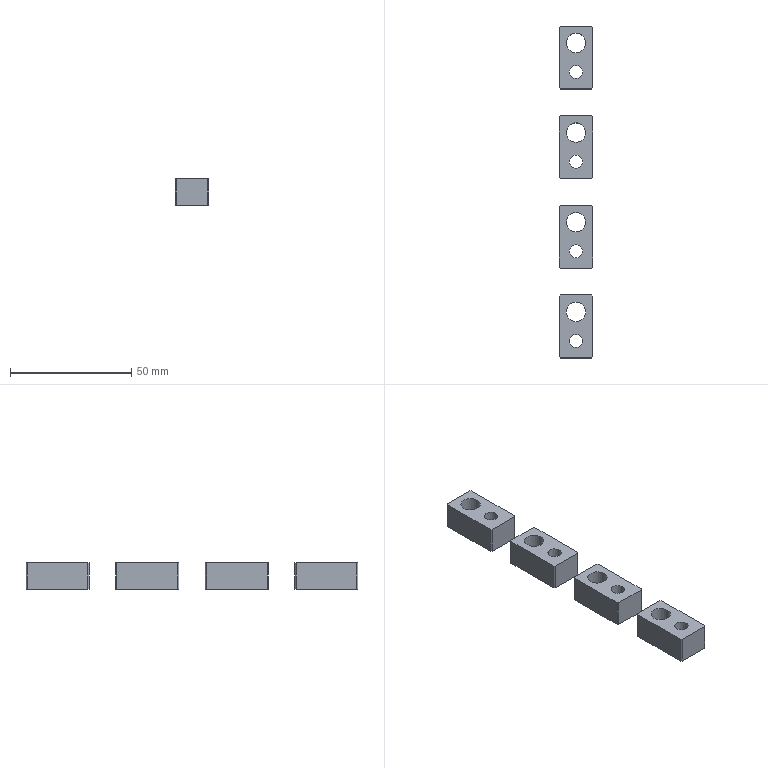CAM job | NX | 3-axis milling, drilling | part box 14 x 137 x 11 mm | stock box 15 x 142 x 15 mm
Tools:
number,name,description,diameter,corner_radius,flute_length,length,flutes
4,D4,平底铣刀-粗,4.0,0.0,25.0,75.0,2
9,D10,平底铣刀-粗,10.0,0.0,35.0,75.0,2
7,D6-J,平底铣刀-精,6.0,0.0,25.0,75.0,2
10,D10-J,平底铣刀-精,10.0,0.0,35.0,75.0,2
1,D80R0.8飞刀,圆鼻刀-粗,80.0,0.8,50.0,75.0,2
2,D6倒角刀,倒角刀,6.0,0.0,3.0,25.0,2
17,钻头5.5,Twist Drill 5 mm,5.5,0.0,52.0,54.0,2
18,ZT7.9,Drilling Tool,7.9,0.0,35.0,50.0,2
Operations:
program,operation,operation_type,tool,method,geometry_group,spindle_rpm,surface_speed,feed_per_tooth,feed_cut,feed_plunge,cut_length_mm,path_length_mm,cut_time_min,machine_time_min
A,顶面,FaceMilling,D80R0.8飞刀,侧刃精光-切深K-步距G,W-A,4000.0,1005.31,0.125,1000.0,100.0,231.0,267.0,0.231,0.2346
A,外形粗_2,VolumeBased25DMillingOperation,D10,METHOD,W-A,8000.0,251.327,0.3125,5000.0,80.0,7102.016,7488.935,1.42,1.459
A,打点-深0.8,Operation,D6倒角刀,NONE,W-A,8000.0,150.796,0.0312,500.0,90.0,14.4,199.026,0.0288,0.0473
A,沉头孔-钻孔0段,Operation,钻头5.5,NONE,W-A,2800.0,48.38,0.0179,100.0,90.0,62.609,279.26,0.6261,0.6478
A,通孔-精孔8.0预钻,Operation,ZT7.9,NONE,W-A,1500.0,37.228,0.0833,250.0,90.0,69.122,292.285,0.2765,0.2988
A,铣孔开粗D4_1,CylinderMilling,D4,NONE,W-A,8000.0,100.531,0.075,1200.0,100.0,1945.99,2297.99,1.622,1.657
A,铣孔精光D4_1,CylinderMilling,D4,精光步距切深关,W-A,8000.0,100.531,0.0312,500.0,100.0,173.186,501.186,0.3464,0.3792
A,仅选体,SurfaceContour,D6倒角刀,METHOD,W-A,8000.0,150.796,0.1875,3000.0,100.0,379.361,636.161,0.1265,0.1521
A,铣倒角_1,PlanarMilling,D6倒角刀,METHOD,W-A,8000.0,150.796,0.0312,500.0,100.0,133.995,423.791,0.268,0.297
A,铣倒角_2,PlanarMilling,D6倒角刀,NONE,W-A,8000.0,150.796,0.0312,500.0,100.0,153.464,419.808,0.3069,0.3336
A,铣孔精光D6-J_1,CylinderMilling,D6-J,精光步距切深关,W-A,8000.0,150.796,0.0187,300.0,100.0,342.669,694.669,1.142,1.177
A,外形半精_2,VolumeBased25DMillingOperation,D10-J,METHOD,W-A,8000.0,251.327,0.0625,1000.0,100.0,469.689,747.199,0.4697,0.4974